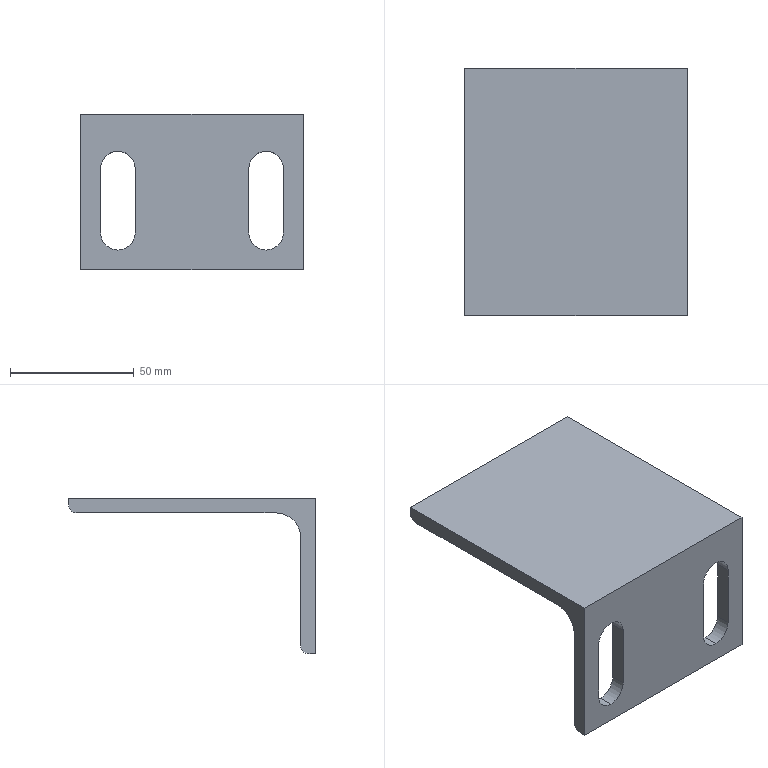Part | STEP file | 03-Counterweight block pressure iron 2_default<machining> | 1 solid | 21 faces | box 90 x 100 x 63 mm | volume 80067 mm3 | plane 12 | cylinder 9 | commonest cylinder face diameters 14 x6 6.667 x2 20 x1